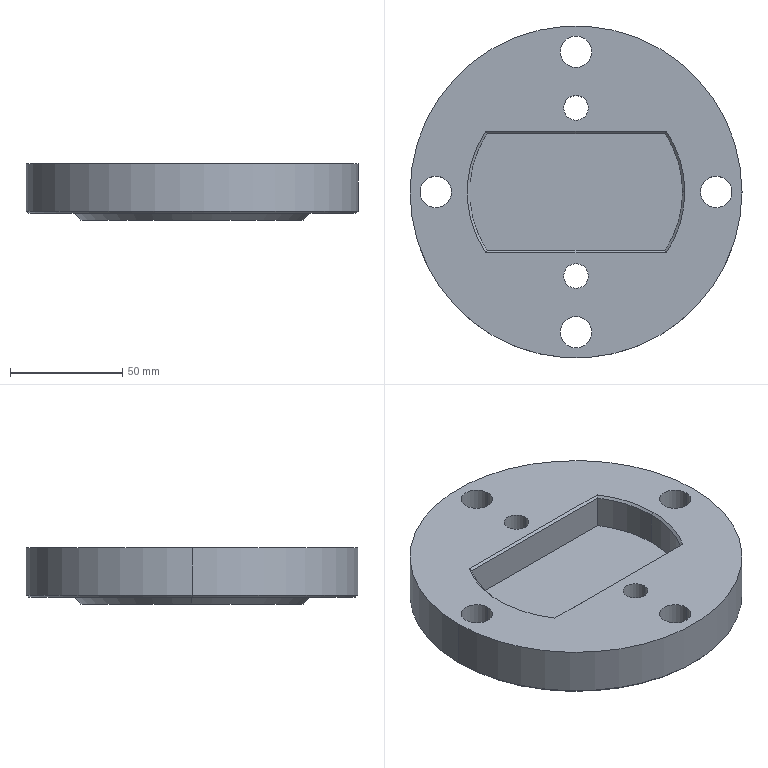Part | SolidWorks | features Chamfer 3, ICE 3, 3DProfileFeature 1, Extrusion 1, HoleWzd 1 | 1 solid | 38 faces | box 148 x 148 x 25 mm | volume 305929 mm3 | cylinder 21 | plane 10 | cone 7 | commonest cylinder face diameters 14 x8 11 x4 18 x4 95 x3 148 x2
STEP:
#1=CARTESIAN_POINT('',(47.5,0.,24.));
#2=VERTEX_POINT('',#1);
#3=CARTESIAN_POINT('',(39.752,26.,24.));
#4=VERTEX_POINT('',#3);
#5=CARTESIAN_POINT('',(0.,0.,24.));
#6=DIRECTION('',(0.,0.,1.));
#7=DIRECTION('',(1.,0.,0.));
#8=AXIS2_PLACEMENT_3D('',#5,#6,#7);
#9=CIRCLE('',#8,47.5);
#10=EDGE_CURVE('',#2,#4,#9,.T.);
#11=ORIENTED_EDGE('',*,*,#10,.F.);
#12=CARTESIAN_POINT('',(48.5,0.,25.));
#13=VERTEX_POINT('',#12);
#14=CARTESIAN_POINT('',(47.5,0.,24.));
#15=DIRECTION('',(0.7071,0.,0.7071));
#16=VECTOR('',#15,1000.);
#17=LINE('',#14,#16);
#18=EDGE_CURVE('',#2,#13,#17,.T.);
#19=ORIENTED_EDGE('',*,*,#18,.T.);
#20=CARTESIAN_POINT('',(40.29,27.,25.));
#21=VERTEX_POINT('',#20);
#22=CARTESIAN_POINT('',(0.,0.,25.));
#23=DIRECTION('',(0.,0.,-1.));
#24=DIRECTION('',(1.,0.,0.));
#25=AXIS2_PLACEMENT_3D('',#22,#23,#24);
#26=CIRCLE('',#25,48.5);
#27=EDGE_CURVE('',#21,#13,#26,.T.);
#28=ORIENTED_EDGE('',*,*,#27,.F.);
#29=CARTESIAN_POINT('',(40.29,27.,25.));
#30=CARTESIAN_POINT('',(40.112,26.666,24.666));
#31=CARTESIAN_POINT('',(39.932,26.333,24.333));
#32=CARTESIAN_POINT('',(39.752,26.,24.));
#33=B_SPLINE_CURVE_WITH_KNOTS('',3,(#29,#30,#31,#32),.UNSPECIFIED.,.F.,.F.,(4,4),(0.,0.001513),.UNSPECIFIED.);
#34=EDGE_CURVE('',#21,#4,#33,.T.);
#35=ORIENTED_EDGE('',*,*,#34,.T.);
#36=EDGE_LOOP('',(#11,#19,#28,#35));
#37=FACE_OUTER_BOUND('',#36,.T.);
#38=CARTESIAN_POINT('',(0.,0.,24.));
#39=DIRECTION('',(0.,0.,1.));
#40=DIRECTION('',(1.,0.,0.));
#41=AXIS2_PLACEMENT_3D('',#38,#39,#40);
#42=CONICAL_SURFACE('',#41,47.5,0.7854);
#43=ADVANCED_FACE('',(#37),#42,.F.);
#44=CARTESIAN_POINT('',(9.,37.5,11.));
#45=VERTEX_POINT('',#44);
#46=CARTESIAN_POINT('',(-9.,37.5,11.));
#47=VERTEX_POINT('',#46);
#48=CARTESIAN_POINT('',(0.,37.5,11.));
#49=DIRECTION('',(0.,0.,-1.));
#50=DIRECTION('',(-1.,0.,0.));
#51=AXIS2_PLACEMENT_3D('',#48,#49,#50);
#52=CIRCLE('',#51,9.);
#53=EDGE_CURVE('',#45,#47,#52,.T.);
#54=ORIENTED_EDGE('',*,*,#53,.F.);
#55=CARTESIAN_POINT('',(9.,37.5,0.));
#56=VERTEX_POINT('',#55);
#57=CARTESIAN_POINT('',(9.,37.5,0.));
#58=DIRECTION('',(0.,0.,-1.));
#59=VECTOR('',#58,1000.);
#60=LINE('',#57,#59);
#61=EDGE_CURVE('',#45,#56,#60,.T.);
#62=ORIENTED_EDGE('',*,*,#61,.T.);
#63=CARTESIAN_POINT('',(-9.,37.5,0.));
#64=VERTEX_POINT('',#63);
#65=CARTESIAN_POINT('',(0.,37.5,0.));
#66=DIRECTION('',(0.,0.,-1.));
#67=DIRECTION('',(-1.,0.,0.));
#68=AXIS2_PLACEMENT_3D('',#65,#66,#67);
#69=CIRCLE('',#68,9.);
#70=EDGE_CURVE('',#56,#64,#69,.T.);
#71=ORIENTED_EDGE('',*,*,#70,.T.);
#72=CARTESIAN_POINT('',(-9.,37.5,0.));
#73=DIRECTION('',(0.,0.,-1.));
#74=VECTOR('',#73,1000.);
#75=LINE('',#72,#74);
#76=EDGE_CURVE('',#47,#64,#75,.T.);
#77=ORIENTED_EDGE('',*,*,#76,.F.);
#78=EDGE_LOOP('',(#54,#62,#71,#77));
#79=FACE_OUTER_BOUND('',#78,.T.);
#80=CARTESIAN_POINT('',(0.,37.5,0.));
#81=DIRECTION('',(0.,0.,-1.));
#82=DIRECTION('',(-1.,0.,0.));
#83=AXIS2_PLACEMENT_3D('',#80,#81,#82);
#84=CYLINDRICAL_SURFACE('',#83,9.);
#85=ADVANCED_FACE('',(#79),#84,.F.);
#86=CARTESIAN_POINT('',(5.5,37.5,25.));
#87=VERTEX_POINT('',#86);
#88=CARTESIAN_POINT('',(-5.5,37.5,25.));
#89=VERTEX_POINT('',#88);
#90=CARTESIAN_POINT('',(0.,37.5,25.));
#91=DIRECTION('',(0.,0.,-1.));
#92=DIRECTION('',(-1.,0.,0.));
#93=AXIS2_PLACEMENT_3D('',#90,#91,#92);
#94=CIRCLE('',#93,5.5);
#95=EDGE_CURVE('',#87,#89,#94,.T.);
#96=ORIENTED_EDGE('',*,*,#95,.F.);
#97=CARTESIAN_POINT('',(5.5,37.5,11.));
#98=VERTEX_POINT('',#97);
#99=CARTESIAN_POINT('',(5.5,37.5,0.));
#100=DIRECTION('',(0.,0.,-1.));
#101=VECTOR('',#100,1000.);
#102=LINE('',#99,#101);
#103=EDGE_CURVE('',#87,#98,#102,.T.);
#104=ORIENTED_EDGE('',*,*,#103,.T.);
#105=CARTESIAN_POINT('',(-5.5,37.5,11.));
#106=VERTEX_POINT('',#105);
#107=CARTESIAN_POINT('',(0.,37.5,11.));
#108=DIRECTION('',(0.,0.,-1.));
#109=DIRECTION('',(-1.,0.,0.));
#110=AXIS2_PLACEMENT_3D('',#107,#108,#109);
#111=CIRCLE('',#110,5.5);
#112=EDGE_CURVE('',#98,#106,#111,.T.);
#113=ORIENTED_EDGE('',*,*,#112,.T.);
#114=CARTESIAN_POINT('',(-5.5,37.5,0.));
#115=DIRECTION('',(0.,0.,-1.));
#116=VECTOR('',#115,1000.);
#117=LINE('',#114,#116);
#118=EDGE_CURVE('',#89,#106,#117,.T.);
#119=ORIENTED_EDGE('',*,*,#118,.F.);
#120=EDGE_LOOP('',(#96,#104,#113,#119));
#121=FACE_OUTER_BOUND('',#120,.T.);
#122=CARTESIAN_POINT('',(0.,37.5,0.));
#123=DIRECTION('',(0.,0.,-1.));
#124=DIRECTION('',(-1.,0.,0.));
#125=AXIS2_PLACEMENT_3D('',#122,#123,#124);
#126=CYLINDRICAL_SURFACE('',#125,5.5);
#127=ADVANCED_FACE('',(#121),#126,.F.);
#128=CARTESIAN_POINT('',(9.,-37.5,11.));
#129=VERTEX_POINT('',#128);
#130=CARTESIAN_POINT('',(-9.,-37.5,11.));
#131=VERTEX_POINT('',#130);
#132=CARTESIAN_POINT('',(0.,-37.5,11.));
#133=DIRECTION('',(0.,0.,-1.));
#134=DIRECTION('',(-1.,0.,0.));
#135=AXIS2_PLACEMENT_3D('',#132,#133,#134);
#136=CIRCLE('',#135,9.);
#137=EDGE_CURVE('',#129,#131,#136,.T.);
#138=ORIENTED_EDGE('',*,*,#137,.F.);
#139=CARTESIAN_POINT('',(9.,-37.5,0.));
#140=VERTEX_POINT('',#139);
#141=CARTESIAN_POINT('',(9.,-37.5,0.));
#142=DIRECTION('',(0.,0.,-1.));
#143=VECTOR('',#142,1000.);
#144=LINE('',#141,#143);
#145=EDGE_CURVE('',#129,#140,#144,.T.);
#146=ORIENTED_EDGE('',*,*,#145,.T.);
#147=CARTESIAN_POINT('',(-9.,-37.5,0.));
#148=VERTEX_POINT('',#147);
#149=CARTESIAN_POINT('',(0.,-37.5,0.));
#150=DIRECTION('',(0.,0.,-1.));
#151=DIRECTION('',(-1.,0.,0.));
#152=AXIS2_PLACEMENT_3D('',#149,#150,#151);
#153=CIRCLE('',#152,9.);
#154=EDGE_CURVE('',#140,#148,#153,.T.);
#155=ORIENTED_EDGE('',*,*,#154,.T.);
#156=CARTESIAN_POINT('',(-9.,-37.5,0.));
#157=DIRECTION('',(0.,0.,-1.));
#158=VECTOR('',#157,1000.);
#159=LINE('',#156,#158);
#160=EDGE_CURVE('',#131,#148,#159,.T.);
#161=ORIENTED_EDGE('',*,*,#160,.F.);
#162=EDGE_LOOP('',(#138,#146,#155,#161));
#163=FACE_OUTER_BOUND('',#162,.T.);
#164=CARTESIAN_POINT('',(0.,-37.5,0.));
#165=DIRECTION('',(0.,0.,-1.));
#166=DIRECTION('',(-1.,0.,0.));
#167=AXIS2_PLACEMENT_3D('',#164,#165,#166);
#168=CYLINDRICAL_SURFACE('',#167,9.);
#169=ADVANCED_FACE('',(#163),#168,.F.);
#170=CARTESIAN_POINT('',(5.5,-37.5,25.));
#171=VERTEX_POINT('',#170);
#172=CARTESIAN_POINT('',(-5.5,-37.5,25.));
#173=VERTEX_POINT('',#172);
#174=CARTESIAN_POINT('',(0.,-37.5,25.));
#175=DIRECTION('',(0.,0.,-1.));
#176=DIRECTION('',(-1.,0.,0.));
#177=AXIS2_PLACEMENT_3D('',#174,#175,#176);
#178=CIRCLE('',#177,5.5);
#179=EDGE_CURVE('',#171,#173,#178,.T.);
#180=ORIENTED_EDGE('',*,*,#179,.F.);
#181=CARTESIAN_POINT('',(5.5,-37.5,11.));
#182=VERTEX_POINT('',#181);
#183=CARTESIAN_POINT('',(5.5,-37.5,0.));
#184=DIRECTION('',(0.,0.,-1.));
#185=VECTOR('',#184,1000.);
#186=LINE('',#183,#185);
#187=EDGE_CURVE('',#171,#182,#186,.T.);
#188=ORIENTED_EDGE('',*,*,#187,.T.);
#189=CARTESIAN_POINT('',(-5.5,-37.5,11.));
#190=VERTEX_POINT('',#189);
#191=CARTESIAN_POINT('',(0.,-37.5,11.));
#192=DIRECTION('',(0.,0.,-1.));
#193=DIRECTION('',(-1.,0.,0.));
#194=AXIS2_PLACEMENT_3D('',#191,#192,#193);
#195=CIRCLE('',#194,5.5);
#196=EDGE_CURVE('',#182,#190,#195,.T.);
#197=ORIENTED_EDGE('',*,*,#196,.T.);
#198=CARTESIAN_POINT('',(-5.5,-37.5,0.));
#199=DIRECTION('',(0.,0.,-1.));
#200=VECTOR('',#199,1000.);
#201=LINE('',#198,#200);
#202=EDGE_CURVE('',#173,#190,#201,.T.);
#203=ORIENTED_EDGE('',*,*,#202,.F.);
#204=EDGE_LOOP('',(#180,#188,#197,#203));
#205=FACE_OUTER_BOUND('',#204,.T.);
#206=CARTESIAN_POINT('',(0.,-37.5,0.));
#207=DIRECTION('',(0.,0.,-1.));
#208=DIRECTION('',(-1.,0.,0.));
#209=AXIS2_PLACEMENT_3D('',#206,#207,#208);
#210=CYLINDRICAL_SURFACE('',#209,5.5);
#211=ADVANCED_FACE('',(#205),#210,.F.);
#212=CARTESIAN_POINT('',(47.5,0.,9.));
#213=VERTEX_POINT('',#212);
#214=CARTESIAN_POINT('',(39.752,26.,9.));
#215=VERTEX_POINT('',#214);
#216=CARTESIAN_POINT('',(0.,0.,9.));
#217=DIRECTION('',(0.,0.,1.));
#218=DIRECTION('',(1.,0.,0.));
#219=AXIS2_PLACEMENT_3D('',#216,#217,#218);
#220=CIRCLE('',#219,47.5);
#221=EDGE_CURVE('',#213,#215,#220,.T.);
#222=ORIENTED_EDGE('',*,*,#221,.F.);
#223=CARTESIAN_POINT('',(47.5,0.,9.));
#224=DIRECTION('',(0.,0.,1.));
#225=VECTOR('',#224,1000.);
#226=LINE('',#223,#225);
#227=EDGE_CURVE('',#213,#2,#226,.T.);
#228=ORIENTED_EDGE('',*,*,#227,.T.);
#229=ORIENTED_EDGE('',*,*,#10,.T.);
#230=CARTESIAN_POINT('',(39.752,26.,9.));
#231=DIRECTION('',(0.,0.,1.));
#232=VECTOR('',#231,1000.);
#233=LINE('',#230,#232);
#234=EDGE_CURVE('',#215,#4,#233,.T.);
#235=ORIENTED_EDGE('',*,*,#234,.F.);
#236=EDGE_LOOP('',(#222,#228,#229,#235));
#237=FACE_OUTER_BOUND('',#236,.T.);
#238=CARTESIAN_POINT('',(0.,0.,9.));
#239=DIRECTION('',(0.,0.,1.));
#240=DIRECTION('',(1.,0.,0.));
#241=AXIS2_PLACEMENT_3D('',#238,#239,#240);
#242=CYLINDRICAL_SURFACE('',#241,47.5);
#243=ADVANCED_FACE('',(#237),#242,.F.);
#244=CARTESIAN_POINT('',(-73.,0.,3.));
#245=VERTEX_POINT('',#244);
#246=CARTESIAN_POINT('',(73.,0.,3.));
#247=VERTEX_POINT('',#246);
#248=CARTESIAN_POINT('',(0.,0.,3.));
#249=DIRECTION('',(0.,0.,-1.));
#250=DIRECTION('',(-1.,0.,0.));
#251=AXIS2_PLACEMENT_3D('',#248,#249,#250);
#252=CIRCLE('',#251,73.);
#253=EDGE_CURVE('',#245,#247,#252,.T.);
#254=ORIENTED_EDGE('',*,*,#253,.F.);
#255=CARTESIAN_POINT('',(-74.,0.,4.));
#256=VERTEX_POINT('',#255);
#257=CARTESIAN_POINT('',(-73.,0.,3.));
#258=DIRECTION('',(-0.7071,0.,0.7071));
#259=VECTOR('',#258,1000.);
#260=LINE('',#257,#259);
#261=EDGE_CURVE('',#245,#256,#260,.T.);
#262=ORIENTED_EDGE('',*,*,#261,.T.);
#263=CARTESIAN_POINT('',(74.,0.,4.));
#264=VERTEX_POINT('',#263);
#265=CARTESIAN_POINT('',(0.,0.,4.));
#266=DIRECTION('',(0.,0.,1.));
#267=DIRECTION('',(-1.,0.,0.));
#268=AXIS2_PLACEMENT_3D('',#265,#266,#267);
#269=CIRCLE('',#268,74.);
#270=EDGE_CURVE('',#264,#256,#269,.T.);
#271=ORIENTED_EDGE('',*,*,#270,.F.);
#272=CARTESIAN_POINT('',(73.,0.,3.));
#273=DIRECTION('',(0.7071,0.,0.7071));
#274=VECTOR('',#273,1000.);
#275=LINE('',#272,#274);
#276=EDGE_CURVE('',#247,#264,#275,.T.);
#277=ORIENTED_EDGE('',*,*,#276,.F.);
#278=EDGE_LOOP('',(#254,#262,#271,#277));
#279=FACE_OUTER_BOUND('',#278,.T.);
#280=CARTESIAN_POINT('',(0.,0.,3.));
#281=DIRECTION('',(0.,0.,1.));
#282=DIRECTION('',(1.,0.,0.));
#283=AXIS2_PLACEMENT_3D('',#280,#281,#282);
#284=CONICAL_SURFACE('',#283,73.,0.7854);
#285=ADVANCED_FACE('',(#279),#284,.T.);
#286=CARTESIAN_POINT('',(-49.5,0.,0.));
#287=VERTEX_POINT('',#286);
#288=CARTESIAN_POINT('',(49.5,0.,0.));
#289=VERTEX_POINT('',#288);
#290=CARTESIAN_POINT('',(0.,0.,0.));
#291=DIRECTION('',(0.,0.,-1.));
#292=DIRECTION('',(1.,0.,0.));
#293=AXIS2_PLACEMENT_3D('',#290,#291,#292);
#294=CIRCLE('',#293,49.5);
#295=EDGE_CURVE('',#287,#289,#294,.T.);
#296=ORIENTED_EDGE('',*,*,#295,.F.);
#297=CARTESIAN_POINT('',(-52.5,0.,3.));
#298=VERTEX_POINT('',#297);
#299=CARTESIAN_POINT('',(-49.5,0.,0.));
#300=DIRECTION('',(-0.7071,0.,0.7071));
#301=VECTOR('',#300,1000.);
#302=LINE('',#299,#301);
#303=EDGE_CURVE('',#287,#298,#302,.T.);
#304=ORIENTED_EDGE('',*,*,#303,.T.);
#305=CARTESIAN_POINT('',(52.5,0.,3.));
#306=VERTEX_POINT('',#305);
#307=CARTESIAN_POINT('',(0.,0.,3.));
#308=DIRECTION('',(0.,0.,-1.));
#309=DIRECTION('',(-1.,0.,0.));
#310=AXIS2_PLACEMENT_3D('',#307,#308,#309);
#311=CIRCLE('',#310,52.5);
#312=EDGE_CURVE('',#298,#306,#311,.T.);
#313=ORIENTED_EDGE('',*,*,#312,.T.);
#314=CARTESIAN_POINT('',(49.5,0.,0.));
#315=DIRECTION('',(0.7071,0.,0.7071));
#316=VECTOR('',#315,1000.);
#317=LINE('',#314,#316);
#318=EDGE_CURVE('',#289,#306,#317,.T.);
#319=ORIENTED_EDGE('',*,*,#318,.F.);
#320=EDGE_LOOP('',(#296,#304,#313,#319));
#321=FACE_OUTER_BOUND('',#320,.T.);
#322=CARTESIAN_POINT('',(0.,0.,0.));
#323=DIRECTION('',(0.,0.,1.));
#324=DIRECTION('',(1.,0.,0.));
#325=AXIS2_PLACEMENT_3D('',#322,#323,#324);
#326=CONICAL_SURFACE('',#325,49.5,0.7854);
#327=ADVANCED_FACE('',(#321),#326,.T.);
#328=CARTESIAN_POINT('',(7.,-62.5,25.));
#329=VERTEX_POINT('',#328);
#330=CARTESIAN_POINT('',(-7.,-62.5,25.));
#331=VERTEX_POINT('',#330);
#332=CARTESIAN_POINT('',(0.,-62.5,25.));
#333=DIRECTION('',(0.,0.,-1.));
#334=DIRECTION('',(-1.,0.,0.));
#335=AXIS2_PLACEMENT_3D('',#332,#333,#334);
#336=CIRCLE('',#335,7.);
#337=EDGE_CURVE('',#329,#331,#336,.T.);
#338=ORIENTED_EDGE('',*,*,#337,.F.);
#339=CARTESIAN_POINT('',(7.,-62.5,3.));
#340=VERTEX_POINT('',#339);
#341=CARTESIAN_POINT('',(7.,-62.5,25.));
#342=DIRECTION('',(0.,0.,-1.));
#343=VECTOR('',#342,1000.);
#344=LINE('',#341,#343);
#345=EDGE_CURVE('',#329,#340,#344,.T.);
#346=ORIENTED_EDGE('',*,*,#345,.T.);
#347=CARTESIAN_POINT('',(-7.,-62.5,3.));
#348=VERTEX_POINT('',#347);
#349=CARTESIAN_POINT('',(0.,-62.5,3.));
#350=DIRECTION('',(0.,0.,-1.));
#351=DIRECTION('',(-1.,0.,0.));
#352=AXIS2_PLACEMENT_3D('',#349,#350,#351);
#353=CIRCLE('',#352,7.);
#354=EDGE_CURVE('',#340,#348,#353,.T.);
#355=ORIENTED_EDGE('',*,*,#354,.T.);
#356=CARTESIAN_POINT('',(-7.,-62.5,25.));
#357=DIRECTION('',(0.,0.,-1.));
#358=VECTOR('',#357,1000.);
#359=LINE('',#356,#358);
#360=EDGE_CURVE('',#331,#348,#359,.T.);
#361=ORIENTED_EDGE('',*,*,#360,.F.);
#362=EDGE_LOOP('',(#338,#346,#355,#361));
#363=FACE_OUTER_BOUND('',#362,.T.);
#364=CARTESIAN_POINT('',(0.,-62.5,25.));
#365=DIRECTION('',(0.,0.,-1.));
#366=DIRECTION('',(-1.,0.,0.));
#367=AXIS2_PLACEMENT_3D('',#364,#365,#366);
#368=CYLINDRICAL_SURFACE('',#367,7.);
#369=ADVANCED_FACE('',(#363),#368,.F.);
#370=CARTESIAN_POINT('',(69.5,0.,25.));
#371=VERTEX_POINT('',#370);
#372=CARTESIAN_POINT('',(55.5,0.,25.));
#373=VERTEX_POINT('',#372);
#374=CARTESIAN_POINT('',(62.5,0.,25.));
#375=DIRECTION('',(0.,0.,-1.));
#376=DIRECTION('',(-1.,0.,0.));
#377=AXIS2_PLACEMENT_3D('',#374,#375,#376);
#378=CIRCLE('',#377,7.);
#379=EDGE_CURVE('',#371,#373,#378,.T.);
#380=ORIENTED_EDGE('',*,*,#379,.F.);
#381=CARTESIAN_POINT('',(69.5,0.,3.));
#382=VERTEX_POINT('',#381);
#383=CARTESIAN_POINT('',(69.5,0.,25.));
#384=DIRECTION('',(0.,0.,-1.));
#385=VECTOR('',#384,1000.);
#386=LINE('',#383,#385);
#387=EDGE_CURVE('',#371,#382,#386,.T.);
#388=ORIENTED_EDGE('',*,*,#387,.T.);
#389=CARTESIAN_POINT('',(55.5,0.,3.));
#390=VERTEX_POINT('',#389);
#391=CARTESIAN_POINT('',(62.5,0.,3.));
#392=DIRECTION('',(0.,0.,-1.));
#393=DIRECTION('',(-1.,0.,0.));
#394=AXIS2_PLACEMENT_3D('',#391,#392,#393);
#395=CIRCLE('',#394,7.);
#396=EDGE_CURVE('',#382,#390,#395,.T.);
#397=ORIENTED_EDGE('',*,*,#396,.T.);
#398=CARTESIAN_POINT('',(55.5,0.,25.));
#399=DIRECTION('',(0.,0.,-1.));
#400=VECTOR('',#399,1000.);
#401=LINE('',#398,#400);
#402=EDGE_CURVE('',#373,#390,#401,.T.);
#403=ORIENTED_EDGE('',*,*,#402,.F.);
#404=EDGE_LOOP('',(#380,#388,#397,#403));
#405=FACE_OUTER_BOUND('',#404,.T.);
#406=CARTESIAN_POINT('',(62.5,0.,25.));
#407=DIRECTION('',(0.,0.,-1.));
#408=DIRECTION('',(-1.,0.,0.));
#409=AXIS2_PLACEMENT_3D('',#406,#407,#408);
#410=CYLINDRICAL_SURFACE('',#409,7.);
#411=ADVANCED_FACE('',(#405),#410,.F.);
#412=CARTESIAN_POINT('',(7.,62.5,25.));
#413=VERTEX_POINT('',#412);
#414=CARTESIAN_POINT('',(-7.,62.5,25.));
#415=VERTEX_POINT('',#414);
#416=CARTESIAN_POINT('',(0.,62.5,25.));
#417=DIRECTION('',(0.,0.,-1.));
#418=DIRECTION('',(-1.,0.,0.));
#419=AXIS2_PLACEMENT_3D('',#416,#417,#418);
#420=CIRCLE('',#419,7.);
#421=EDGE_CURVE('',#413,#415,#420,.T.);
#422=ORIENTED_EDGE('',*,*,#421,.F.);
#423=CARTESIAN_POINT('',(7.,62.5,3.));
#424=VERTEX_POINT('',#423);
#425=CARTESIAN_POINT('',(7.,62.5,25.));
#426=DIRECTION('',(0.,0.,-1.));
#427=VECTOR('',#426,1000.);
#428=LINE('',#425,#427);
#429=EDGE_CURVE('',#413,#424,#428,.T.);
#430=ORIENTED_EDGE('',*,*,#429,.T.);
#431=CARTESIAN_POINT('',(-7.,62.5,3.));
#432=VERTEX_POINT('',#431);
#433=CARTESIAN_POINT('',(0.,62.5,3.));
#434=DIRECTION('',(0.,0.,-1.));
#435=DIRECTION('',(-1.,0.,0.));
#436=AXIS2_PLACEMENT_3D('',#433,#434,#435);
#437=CIRCLE('',#436,7.);
#438=EDGE_CURVE('',#424,#432,#437,.T.);
#439=ORIENTED_EDGE('',*,*,#438,.T.);
#440=CARTESIAN_POINT('',(-7.,62.5,25.));
#441=DIRECTION('',(0.,0.,-1.));
#442=VECTOR('',#441,1000.);
#443=LINE('',#440,#442);
#444=EDGE_CURVE('',#415,#432,#443,.T.);
#445=ORIENTED_EDGE('',*,*,#444,.F.);
#446=EDGE_LOOP('',(#422,#430,#439,#445));
#447=FACE_OUTER_BOUND('',#446,.T.);
#448=CARTESIAN_POINT('',(0.,62.5,25.));
#449=DIRECTION('',(0.,0.,-1.));
#450=DIRECTION('',(-1.,0.,0.));
#451=AXIS2_PLACEMENT_3D('',#448,#449,#450);
#452=CYLINDRICAL_SURFACE('',#451,7.);
#453=ADVANCED_FACE('',(#447),#452,.F.);
#454=CARTESIAN_POINT('',(-55.5,0.,25.));
#455=VERTEX_POINT('',#454);
#456=CARTESIAN_POINT('',(-69.5,0.,25.));
#457=VERTEX_POINT('',#456);
#458=CARTESIAN_POINT('',(-62.5,0.,25.));
#459=DIRECTION('',(0.,0.,-1.));
#460=DIRECTION('',(-1.,0.,0.));
#461=AXIS2_PLACEMENT_3D('',#458,#459,#460);
#462=CIRCLE('',#461,7.);
#463=EDGE_CURVE('',#455,#457,#462,.T.);
#464=ORIENTED_EDGE('',*,*,#463,.F.);
#465=CARTESIAN_POINT('',(-55.5,0.,3.));
#466=VERTEX_POINT('',#465);
#467=CARTESIAN_POINT('',(-55.5,0.,25.));
#468=DIRECTION('',(0.,0.,-1.));
#469=VECTOR('',#468,1000.);
#470=LINE('',#467,#469);
#471=EDGE_CURVE('',#455,#466,#470,.T.);
#472=ORIENTED_EDGE('',*,*,#471,.T.);
#473=CARTESIAN_POINT('',(-69.5,0.,3.));
#474=VERTEX_POINT('',#473);
#475=CARTESIAN_POINT('',(-62.5,0.,3.));
#476=DIRECTION('',(0.,0.,-1.));
#477=DIRECTION('',(-1.,0.,0.));
#478=AXIS2_PLACEMENT_3D('',#475,#476,#477);
#479=CIRCLE('',#478,7.);
#480=EDGE_CURVE('',#466,#474,#479,.T.);
#481=ORIENTED_EDGE('',*,*,#480,.T.);
#482=CARTESIAN_POINT('',(-69.5,0.,25.));
#483=DIRECTION('',(0.,0.,-1.));
#484=VECTOR('',#483,1000.);
#485=LINE('',#482,#484);
#486=EDGE_CURVE('',#457,#474,#485,.T.);
#487=ORIENTED_EDGE('',*,*,#486,.F.);
#488=EDGE_LOOP('',(#464,#472,#481,#487));
#489=FACE_OUTER_BOUND('',#488,.T.);
#490=CARTESIAN_POINT('',(-62.5,0.,25.));
#491=DIRECTION('',(0.,0.,-1.));
#492=DIRECTION('',(-1.,0.,0.));
#493=AXIS2_PLACEMENT_3D('',#490,#491,#492);
#494=CYLINDRICAL_SURFACE('',#493,7.);
#495=ADVANCED_FACE('',(#489),#494,.F.);
#496=CARTESIAN_POINT('',(74.,0.,25.));
#497=VERTEX_POINT('',#496);
#498=CARTESIAN_POINT('',(-74.,0.,25.));
#499=VERTEX_POINT('',#498);
#500=CARTESIAN_POINT('',(0.,0.,25.));
#501=DIRECTION('',(0.,0.,1.));
#502=DIRECTION('',(1.,0.,0.));
#503=AXIS2_PLACEMENT_3D('',#500,#501,#502);
#504=CIRCLE('',#503,74.);
#505=EDGE_CURVE('',#497,#499,#504,.T.);
#506=ORIENTED_EDGE('',*,*,#505,.F.);
#507=CARTESIAN_POINT('',(74.,0.,25.));
#508=DIRECTION('',(0.,0.,-1.));
#509=VECTOR('',#508,1000.);
#510=LINE('',#507,#509);
#511=EDGE_CURVE('',#497,#264,#510,.T.);
#512=ORIENTED_EDGE('',*,*,#511,.T.);
#513=ORIENTED_EDGE('',*,*,#270,.T.);
#514=CARTESIAN_POINT('',(-74.,0.,25.));
#515=DIRECTION('',(0.,0.,-1.));
#516=VECTOR('',#515,1000.);
#517=LINE('',#514,#516);
#518=EDGE_CURVE('',#499,#256,#517,.T.);
#519=ORIENTED_EDGE('',*,*,#518,.F.);
#520=EDGE_LOOP('',(#506,#512,#513,#519));
#521=FACE_OUTER_BOUND('',#520,.T.);
#522=CARTESIAN_POINT('',(0.,0.,25.));
#523=DIRECTION('',(0.,0.,-1.));
#524=DIRECTION('',(-1.,0.,0.));
#525=AXIS2_PLACEMENT_3D('',#522,#523,#524);
#526=CYLINDRICAL_SURFACE('',#525,74.);
#527=ADVANCED_FACE('',(#521),#526,.T.);
#528=ORIENTED_EDGE('',*,*,#511,.F.);
#529=CARTESIAN_POINT('',(0.,0.,25.));
#530=DIRECTION('',(0.,0.,1.));
#531=DIRECTION('',(1.,0.,0.));
#532=AXIS2_PLACEMENT_3D('',#529,#530,#531);
#533=CIRCLE('',#532,74.);
#534=EDGE_CURVE('',#499,#497,#533,.T.);
#535=ORIENTED_EDGE('',*,*,#534,.F.);
#536=ORIENTED_EDGE('',*,*,#518,.T.);
#537=CARTESIAN_POINT('',(0.,0.,4.));
#538=DIRECTION('',(0.,0.,1.));
#539=DIRECTION('',(-1.,0.,0.));
#540=AXIS2_PLACEMENT_3D('',#537,#538,#539);
#541=CIRCLE('',#540,74.);
#542=EDGE_CURVE('',#256,#264,#541,.T.);
#543=ORIENTED_EDGE('',*,*,#542,.T.);
#544=EDGE_LOOP('',(#528,#535,#536,#543));
#545=FACE_OUTER_BOUND('',#544,.T.);
#546=CARTESIAN_POINT('',(0.,0.,25.));
#547=DIRECTION('',(0.,0.,-1.));
#548=DIRECTION('',(-1.,0.,0.));
#549=AXIS2_PLACEMENT_3D('',#546,#547,#548);
#550=CYLINDRICAL_SURFACE('',#549,74.);
#551=ADVANCED_FACE('',(#545),#550,.T.);
#552=CARTESIAN_POINT('',(-40.29,27.,25.));
#553=VERTEX_POINT('',#552);
#554=CARTESIAN_POINT('',(39.752,27.,25.));
#555=DIRECTION('',(1.,0.,0.));
#556=VECTOR('',#555,1000.);
#557=LINE('',#554,#556);
#558=EDGE_CURVE('',#553,#21,#557,.T.);
#559=ORIENTED_EDGE('',*,*,#558,.T.);
#560=ORIENTED_EDGE('',*,*,#27,.T.);
#561=CARTESIAN_POINT('',(40.29,-27.,25.));
#562=VERTEX_POINT('',#561);
#563=CARTESIAN_POINT('',(0.,0.,25.));
#564=DIRECTION('',(0.,0.,-1.));
#565=DIRECTION('',(1.,0.,0.));
#566=AXIS2_PLACEMENT_3D('',#563,#564,#565);
#567=CIRCLE('',#566,48.5);
#568=EDGE_CURVE('',#13,#562,#567,.T.);
#569=ORIENTED_EDGE('',*,*,#568,.T.);
#570=CARTESIAN_POINT('',(-40.29,-27.,25.));
#571=VERTEX_POINT('',#570);
#572=CARTESIAN_POINT('',(-39.752,-27.,25.));
#573=DIRECTION('',(-1.,0.,0.));
#574=VECTOR('',#573,1000.);
#575=LINE('',#572,#574);
#576=EDGE_CURVE('',#562,#571,#575,.T.);
#577=ORIENTED_EDGE('',*,*,#576,.T.);
#578=CARTESIAN_POINT('',(0.,0.,25.));
#579=DIRECTION('',(0.,0.,-1.));
#580=DIRECTION('',(1.,0.,0.));
#581=AXIS2_PLACEMENT_3D('',#578,#579,#580);
#582=CIRCLE('',#581,48.5);
#583=EDGE_CURVE('',#571,#553,#582,.T.);
#584=ORIENTED_EDGE('',*,*,#583,.T.);
#585=EDGE_LOOP('',(#559,#560,#569,#577,#584));
#586=FACE_BOUND('',#585,.T.);
#587=CARTESIAN_POINT('',(0.,37.5,25.));
#588=DIRECTION('',(0.,0.,-1.));
#589=DIRECTION('',(-1.,0.,0.));
#590=AXIS2_PLACEMENT_3D('',#587,#588,#589);
#591=CIRCLE('',#590,5.5);
#592=EDGE_CURVE('',#89,#87,#591,.T.);
#593=ORIENTED_EDGE('',*,*,#592,.T.);
#594=ORIENTED_EDGE('',*,*,#95,.T.);
#595=EDGE_LOOP('',(#593,#594));
#596=FACE_BOUND('',#595,.T.);
#597=CARTESIAN_POINT('',(0.,-37.5,25.));
#598=DIRECTION('',(0.,0.,-1.));
#599=DIRECTION('',(-1.,0.,0.));
#600=AXIS2_PLACEMENT_3D('',#597,#598,#599);
#601=CIRCLE('',#600,5.5);
#602=EDGE_CURVE('',#173,#171,#601,.T.);
#603=ORIENTED_EDGE('',*,*,#602,.T.);
#604=ORIENTED_EDGE('',*,*,#179,.T.);
#605=EDGE_LOOP('',(#603,#604));
#606=FACE_BOUND('',#605,.T.);
#607=CARTESIAN_POINT('',(0.,-62.5,25.));
#608=DIRECTION('',(0.,0.,-1.));
#609=DIRECTION('',(-1.,0.,0.));
#610=AXIS2_PLACEMENT_3D('',#607,#608,#609);
#611=CIRCLE('',#610,7.);
#612=EDGE_CURVE('',#331,#329,#611,.T.);
#613=ORIENTED_EDGE('',*,*,#612,.T.);
#614=ORIENTED_EDGE('',*,*,#337,.T.);
#615=EDGE_LOOP('',(#613,#614));
#616=FACE_BOUND('',#615,.T.);
#617=CARTESIAN_POINT('',(62.5,0.,25.));
#618=DIRECTION('',(0.,0.,-1.));
#619=DIRECTION('',(-1.,0.,0.));
#620=AXIS2_PLACEMENT_3D('',#617,#618,#619);
#621=CIRCLE('',#620,7.);
#622=EDGE_CURVE('',#373,#371,#621,.T.);
#623=ORIENTED_EDGE('',*,*,#622,.T.);
#624=ORIENTED_EDGE('',*,*,#379,.T.);
#625=EDGE_LOOP('',(#623,#624));
#626=FACE_BOUND('',#625,.T.);
#627=CARTESIAN_POINT('',(0.,62.5,25.));
#628=DIRECTION('',(0.,0.,-1.));
#629=DIRECTION('',(-1.,0.,0.));
#630=AXIS2_PLACEMENT_3D('',#627,#628,#629);
#631=CIRCLE('',#630,7.);
#632=EDGE_CURVE('',#415,#413,#631,.T.);
#633=ORIENTED_EDGE('',*,*,#632,.T.);
#634=ORIENTED_EDGE('',*,*,#421,.T.);
#635=EDGE_LOOP('',(#633,#634));
#636=FACE_BOUND('',#635,.T.);
#637=CARTESIAN_POINT('',(-62.5,0.,25.));
#638=DIRECTION('',(0.,0.,-1.));
#639=DIRECTION('',(-1.,0.,0.));
#640=AXIS2_PLACEMENT_3D('',#637,#638,#639);
#641=CIRCLE('',#640,7.);
#642=EDGE_CURVE('',#457,#455,#641,.T.);
#643=ORIENTED_EDGE('',*,*,#642,.T.);
#644=ORIENTED_EDGE('',*,*,#463,.T.);
#645=EDGE_LOOP('',(#643,#644));
#646=FACE_BOUND('',#645,.T.);
#647=ORIENTED_EDGE('',*,*,#534,.T.);
#648=ORIENTED_EDGE('',*,*,#505,.T.);
#649=EDGE_LOOP('',(#647,#648));
#650=FACE_OUTER_BOUND('',#649,.T.);
#651=CARTESIAN_POINT('',(0.,0.,25.));
#652=DIRECTION('',(0.,0.,1.));
#653=DIRECTION('',(1.,0.,0.));
#654=AXIS2_PLACEMENT_3D('',#651,#652,#653);
#655=PLANE('',#654);
#656=ADVANCED_FACE('',(#586,#596,#606,#616,#626,#636,#646,#650),#655,.T.);
#657=CARTESIAN_POINT('',(0.,0.,3.));
#658=DIRECTION('',(0.,0.,-1.));
#659=DIRECTION('',(-1.,0.,0.));
#660=AXIS2_PLACEMENT_3D('',#657,#658,#659);
#661=CIRCLE('',#660,73.);
#662=EDGE_CURVE('',#247,#245,#661,.T.);
#663=ORIENTED_EDGE('',*,*,#662,.T.);
#664=ORIENTED_EDGE('',*,*,#253,.T.);
#665=EDGE_LOOP('',(#663,#664));
#666=FACE_OUTER_BOUND('',#665,.T.);
#667=CARTESIAN_POINT('',(0.,-62.5,3.));
#668=DIRECTION('',(0.,0.,-1.));
#669=DIRECTION('',(-1.,0.,0.));
#670=AXIS2_PLACEMENT_3D('',#667,#668,#669);
#671=CIRCLE('',#670,7.);
#672=EDGE_CURVE('',#348,#340,#671,.T.);
#673=ORIENTED_EDGE('',*,*,#672,.F.);
#674=ORIENTED_EDGE('',*,*,#354,.F.);
#675=EDGE_LOOP('',(#673,#674));
#676=FACE_BOUND('',#675,.T.);
#677=CARTESIAN_POINT('',(62.5,0.,3.));
#678=DIRECTION('',(0.,0.,-1.));
#679=DIRECTION('',(-1.,0.,0.));
#680=AXIS2_PLACEMENT_3D('',#677,#678,#679);
#681=CIRCLE('',#680,7.);
#682=EDGE_CURVE('',#390,#382,#681,.T.);
#683=ORIENTED_EDGE('',*,*,#682,.F.);
#684=ORIENTED_EDGE('',*,*,#396,.F.);
#685=EDGE_LOOP('',(#683,#684));
#686=FACE_BOUND('',#685,.T.);
#687=CARTESIAN_POINT('',(0.,62.5,3.));
#688=DIRECTION('',(0.,0.,-1.));
#689=DIRECTION('',(-1.,0.,0.));
#690=AXIS2_PLACEMENT_3D('',#687,#688,#689);
#691=CIRCLE('',#690,7.);
#692=EDGE_CURVE('',#432,#424,#691,.T.);
#693=ORIENTED_EDGE('',*,*,#692,.F.);
#694=ORIENTED_EDGE('',*,*,#438,.F.);
#695=EDGE_LOOP('',(#693,#694));
#696=FACE_BOUND('',#695,.T.);
#697=CARTESIAN_POINT('',(-62.5,0.,3.));
#698=DIRECTION('',(0.,0.,-1.));
#699=DIRECTION('',(-1.,0.,0.));
#700=AXIS2_PLACEMENT_3D('',#697,#698,#699);
#701=CIRCLE('',#700,7.);
#702=EDGE_CURVE('',#474,#466,#701,.T.);
#703=ORIENTED_EDGE('',*,*,#702,.F.);
#704=ORIENTED_EDGE('',*,*,#480,.F.);
#705=EDGE_LOOP('',(#703,#704));
#706=FACE_BOUND('',#705,.T.);
#707=CARTESIAN_POINT('',(0.,0.,3.));
#708=DIRECTION('',(0.,0.,-1.));
#709=DIRECTION('',(-1.,0.,0.));
#710=AXIS2_PLACEMENT_3D('',#707,#708,#709);
#711=CIRCLE('',#710,52.5);
#712=EDGE_CURVE('',#306,#298,#711,.T.);
#713=ORIENTED_EDGE('',*,*,#712,.F.);
#714=ORIENTED_EDGE('',*,*,#312,.F.);
#715=EDGE_LOOP('',(#713,#714));
#716=FACE_BOUND('',#715,.T.);
#717=CARTESIAN_POINT('',(0.,0.,3.));
#718=DIRECTION('',(0.,0.,-1.));
#719=DIRECTION('',(-1.,0.,0.));
#720=AXIS2_PLACEMENT_3D('',#717,#718,#719);
#721=PLANE('',#720);
#722=ADVANCED_FACE('',(#666,#676,#686,#696,#706,#716),#721,.T.);
#723=CARTESIAN_POINT('',(0.,37.5,0.));
#724=DIRECTION('',(0.,0.,-1.));
#725=DIRECTION('',(-1.,0.,0.));
#726=AXIS2_PLACEMENT_3D('',#723,#724,#725);
#727=CIRCLE('',#726,9.);
#728=EDGE_CURVE('',#64,#56,#727,.T.);
#729=ORIENTED_EDGE('',*,*,#728,.F.);
#730=ORIENTED_EDGE('',*,*,#70,.F.);
#731=EDGE_LOOP('',(#729,#730));
#732=FACE_BOUND('',#731,.T.);
#733=CARTESIAN_POINT('',(0.,-37.5,0.));
#734=DIRECTION('',(0.,0.,-1.));
#735=DIRECTION('',(-1.,0.,0.));
#736=AXIS2_PLACEMENT_3D('',#733,#734,#735);
#737=CIRCLE('',#736,9.);
#738=EDGE_CURVE('',#148,#140,#737,.T.);
#739=ORIENTED_EDGE('',*,*,#738,.F.);
#740=ORIENTED_EDGE('',*,*,#154,.F.);
#741=EDGE_LOOP('',(#739,#740));
#742=FACE_BOUND('',#741,.T.);
#743=CARTESIAN_POINT('',(0.,0.,0.));
#744=DIRECTION('',(0.,0.,-1.));
#745=DIRECTION('',(1.,0.,0.));
#746=AXIS2_PLACEMENT_3D('',#743,#744,#745);
#747=CIRCLE('',#746,49.5);
#748=EDGE_CURVE('',#289,#287,#747,.T.);
#749=ORIENTED_EDGE('',*,*,#748,.T.);
#750=ORIENTED_EDGE('',*,*,#295,.T.);
#751=EDGE_LOOP('',(#749,#750));
#752=FACE_OUTER_BOUND('',#751,.T.);
#753=CARTESIAN_POINT('',(0.,0.,0.));
#754=DIRECTION('',(0.,0.,1.));
#755=DIRECTION('',(1.,0.,0.));
#756=AXIS2_PLACEMENT_3D('',#753,#754,#755);
#757=PLANE('',#756);
#758=ADVANCED_FACE('',(#732,#742,#752),#757,.F.);
#759=ORIENTED_EDGE('',*,*,#471,.F.);
#760=ORIENTED_EDGE('',*,*,#642,.F.);
#761=ORIENTED_EDGE('',*,*,#486,.T.);
#762=ORIENTED_EDGE('',*,*,#702,.T.);
#763=EDGE_LOOP('',(#759,#760,#761,#762));
#764=FACE_OUTER_BOUND('',#763,.T.);
#765=CARTESIAN_POINT('',(-62.5,0.,25.));
#766=DIRECTION('',(0.,0.,-1.));
#767=DIRECTION('',(-1.,0.,0.));
#768=AXIS2_PLACEMENT_3D('',#765,#766,#767);
#769=CYLINDRICAL_SURFACE('',#768,7.);
#770=ADVANCED_FACE('',(#764),#769,.F.);
#771=ORIENTED_EDGE('',*,*,#429,.F.);
#772=ORIENTED_EDGE('',*,*,#632,.F.);
#773=ORIENTED_EDGE('',*,*,#444,.T.);
#774=ORIENTED_EDGE('',*,*,#692,.T.);
#775=EDGE_LOOP('',(#771,#772,#773,#774));
#776=FACE_OUTER_BOUND('',#775,.T.);
#777=CARTESIAN_POINT('',(0.,62.5,25.));
#778=DIRECTION('',(0.,0.,-1.));
#779=DIRECTION('',(-1.,0.,0.));
#780=AXIS2_PLACEMENT_3D('',#777,#778,#779);
#781=CYLINDRICAL_SURFACE('',#780,7.);
#782=ADVANCED_FACE('',(#776),#781,.F.);
#783=ORIENTED_EDGE('',*,*,#387,.F.);
#784=ORIENTED_EDGE('',*,*,#622,.F.);
#785=ORIENTED_EDGE('',*,*,#402,.T.);
#786=ORIENTED_EDGE('',*,*,#682,.T.);
#787=EDGE_LOOP('',(#783,#784,#785,#786));
#788=FACE_OUTER_BOUND('',#787,.T.);
#789=CARTESIAN_POINT('',(62.5,0.,25.));
#790=DIRECTION('',(0.,0.,-1.));
#791=DIRECTION('',(-1.,0.,0.));
#792=AXIS2_PLACEMENT_3D('',#789,#790,#791);
#793=CYLINDRICAL_SURFACE('',#792,7.);
#794=ADVANCED_FACE('',(#788),#793,.F.);
#795=ORIENTED_EDGE('',*,*,#345,.F.);
#796=ORIENTED_EDGE('',*,*,#612,.F.);
#797=ORIENTED_EDGE('',*,*,#360,.T.);
#798=ORIENTED_EDGE('',*,*,#672,.T.);
#799=EDGE_LOOP('',(#795,#796,#797,#798));
#800=FACE_OUTER_BOUND('',#799,.T.);
#801=CARTESIAN_POINT('',(0.,-62.5,25.));
#802=DIRECTION('',(0.,0.,-1.));
#803=DIRECTION('',(-1.,0.,0.));
#804=AXIS2_PLACEMENT_3D('',#801,#802,#803);
#805=CYLINDRICAL_SURFACE('',#804,7.);
#806=ADVANCED_FACE('',(#800),#805,.F.);
#807=ORIENTED_EDGE('',*,*,#303,.F.);
#808=ORIENTED_EDGE('',*,*,#748,.F.);
#809=ORIENTED_EDGE('',*,*,#318,.T.);
#810=ORIENTED_EDGE('',*,*,#712,.T.);
#811=EDGE_LOOP('',(#807,#808,#809,#810));
#812=FACE_OUTER_BOUND('',#811,.T.);
#813=CARTESIAN_POINT('',(0.,0.,0.));
#814=DIRECTION('',(0.,0.,1.));
#815=DIRECTION('',(1.,0.,0.));
#816=AXIS2_PLACEMENT_3D('',#813,#814,#815);
#817=CONICAL_SURFACE('',#816,49.5,0.7854);
#818=ADVANCED_FACE('',(#812),#817,.T.);
#819=ORIENTED_EDGE('',*,*,#261,.F.);
#820=ORIENTED_EDGE('',*,*,#662,.F.);
#821=ORIENTED_EDGE('',*,*,#276,.T.);
#822=ORIENTED_EDGE('',*,*,#542,.F.);
#823=EDGE_LOOP('',(#819,#820,#821,#822));
#824=FACE_OUTER_BOUND('',#823,.T.);
#825=CARTESIAN_POINT('',(0.,0.,3.));
#826=DIRECTION('',(0.,0.,1.));
#827=DIRECTION('',(1.,0.,0.));
#828=AXIS2_PLACEMENT_3D('',#825,#826,#827);
#829=CONICAL_SURFACE('',#828,73.,0.7854);
#830=ADVANCED_FACE('',(#824),#829,.T.);
#831=CARTESIAN_POINT('',(-39.752,26.,9.));
#832=VERTEX_POINT('',#831);
#833=CARTESIAN_POINT('',(-39.752,26.,24.));
#834=VERTEX_POINT('',#833);
#835=CARTESIAN_POINT('',(-39.752,26.,9.));
#836=DIRECTION('',(0.,0.,1.));
#837=VECTOR('',#836,1000.);
#838=LINE('',#835,#837);
#839=EDGE_CURVE('',#832,#834,#838,.T.);
#840=ORIENTED_EDGE('',*,*,#839,.T.);
#841=CARTESIAN_POINT('',(-39.752,-26.,24.));
#842=VERTEX_POINT('',#841);
#843=CARTESIAN_POINT('',(0.,0.,24.));
#844=DIRECTION('',(0.,0.,1.));
#845=DIRECTION('',(1.,0.,0.));
#846=AXIS2_PLACEMENT_3D('',#843,#844,#845);
#847=CIRCLE('',#846,47.5);
#848=EDGE_CURVE('',#834,#842,#847,.T.);
#849=ORIENTED_EDGE('',*,*,#848,.T.);
#850=CARTESIAN_POINT('',(-39.752,-26.,9.));
#851=VERTEX_POINT('',#850);
#852=CARTESIAN_POINT('',(-39.752,-26.,9.));
#853=DIRECTION('',(0.,0.,1.));
#854=VECTOR('',#853,1000.);
#855=LINE('',#852,#854);
#856=EDGE_CURVE('',#851,#842,#855,.T.);
#857=ORIENTED_EDGE('',*,*,#856,.F.);
#858=CARTESIAN_POINT('',(0.,0.,9.));
#859=DIRECTION('',(0.,0.,1.));
#860=DIRECTION('',(1.,0.,0.));
#861=AXIS2_PLACEMENT_3D('',#858,#859,#860);
#862=CIRCLE('',#861,47.5);
#863=EDGE_CURVE('',#832,#851,#862,.T.);
#864=ORIENTED_EDGE('',*,*,#863,.F.);
#865=EDGE_LOOP('',(#840,#849,#857,#864));
#866=FACE_OUTER_BOUND('',#865,.T.);
#867=CARTESIAN_POINT('',(0.,0.,9.));
#868=DIRECTION('',(0.,0.,1.));
#869=DIRECTION('',(1.,0.,0.));
#870=AXIS2_PLACEMENT_3D('',#867,#868,#869);
#871=CYLINDRICAL_SURFACE('',#870,47.5);
#872=ADVANCED_FACE('',(#866),#871,.F.);
#873=ORIENTED_EDGE('',*,*,#234,.T.);
#874=CARTESIAN_POINT('',(-39.752,26.,24.));
#875=DIRECTION('',(-1.,0.,0.));
#876=VECTOR('',#875,1000.);
#877=LINE('',#874,#876);
#878=EDGE_CURVE('',#4,#834,#877,.T.);
#879=ORIENTED_EDGE('',*,*,#878,.T.);
#880=ORIENTED_EDGE('',*,*,#839,.F.);
#881=CARTESIAN_POINT('',(-39.752,26.,9.));
#882=DIRECTION('',(-1.,0.,0.));
#883=VECTOR('',#882,1000.);
#884=LINE('',#881,#883);
#885=EDGE_CURVE('',#215,#832,#884,.T.);
#886=ORIENTED_EDGE('',*,*,#885,.F.);
#887=EDGE_LOOP('',(#873,#879,#880,#886));
#888=FACE_OUTER_BOUND('',#887,.T.);
#889=CARTESIAN_POINT('',(-39.752,26.,9.));
#890=DIRECTION('',(0.,1.,0.));
#891=DIRECTION('',(0.,0.,1.));
#892=AXIS2_PLACEMENT_3D('',#889,#890,#891);
#893=PLANE('',#892);
#894=ADVANCED_FACE('',(#888),#893,.F.);
#895=ORIENTED_EDGE('',*,*,#227,.F.);
#896=CARTESIAN_POINT('',(39.752,-26.,9.));
#897=VERTEX_POINT('',#896);
#898=CARTESIAN_POINT('',(0.,0.,9.));
#899=DIRECTION('',(0.,0.,1.));
#900=DIRECTION('',(1.,0.,0.));
#901=AXIS2_PLACEMENT_3D('',#898,#899,#900);
#902=CIRCLE('',#901,47.5);
#903=EDGE_CURVE('',#897,#213,#902,.T.);
#904=ORIENTED_EDGE('',*,*,#903,.F.);
#905=CARTESIAN_POINT('',(39.752,-26.,24.));
#906=VERTEX_POINT('',#905);
#907=CARTESIAN_POINT('',(39.752,-26.,9.));
#908=DIRECTION('',(0.,0.,1.));
#909=VECTOR('',#908,1000.);
#910=LINE('',#907,#909);
#911=EDGE_CURVE('',#897,#906,#910,.T.);
#912=ORIENTED_EDGE('',*,*,#911,.T.);
#913=CARTESIAN_POINT('',(0.,0.,24.));
#914=DIRECTION('',(0.,0.,1.));
#915=DIRECTION('',(1.,0.,0.));
#916=AXIS2_PLACEMENT_3D('',#913,#914,#915);
#917=CIRCLE('',#916,47.5);
#918=EDGE_CURVE('',#906,#2,#917,.T.);
#919=ORIENTED_EDGE('',*,*,#918,.T.);
#920=EDGE_LOOP('',(#895,#904,#912,#919));
#921=FACE_OUTER_BOUND('',#920,.T.);
#922=CARTESIAN_POINT('',(0.,0.,9.));
#923=DIRECTION('',(0.,0.,1.));
#924=DIRECTION('',(1.,0.,0.));
#925=AXIS2_PLACEMENT_3D('',#922,#923,#924);
#926=CYLINDRICAL_SURFACE('',#925,47.5);
#927=ADVANCED_FACE('',(#921),#926,.F.);
#928=ORIENTED_EDGE('',*,*,#856,.T.);
#929=CARTESIAN_POINT('',(39.752,-26.,24.));
#930=DIRECTION('',(1.,0.,0.));
#931=VECTOR('',#930,1000.);
#932=LINE('',#929,#931);
#933=EDGE_CURVE('',#842,#906,#932,.T.);
#934=ORIENTED_EDGE('',*,*,#933,.T.);
#935=ORIENTED_EDGE('',*,*,#911,.F.);
#936=CARTESIAN_POINT('',(-39.752,-26.,9.));
#937=DIRECTION('',(1.,0.,0.));
#938=VECTOR('',#937,1000.);
#939=LINE('',#936,#938);
#940=EDGE_CURVE('',#851,#897,#939,.T.);
#941=ORIENTED_EDGE('',*,*,#940,.F.);
#942=EDGE_LOOP('',(#928,#934,#935,#941));
#943=FACE_OUTER_BOUND('',#942,.T.);
#944=CARTESIAN_POINT('',(-39.752,-26.,9.));
#945=DIRECTION('',(0.,-1.,0.));
#946=DIRECTION('',(0.,0.,-1.));
#947=AXIS2_PLACEMENT_3D('',#944,#945,#946);
#948=PLANE('',#947);
#949=ADVANCED_FACE('',(#943),#948,.F.);
#950=ORIENTED_EDGE('',*,*,#863,.T.);
#951=ORIENTED_EDGE('',*,*,#940,.T.);
#952=ORIENTED_EDGE('',*,*,#903,.T.);
#953=ORIENTED_EDGE('',*,*,#221,.T.);
#954=ORIENTED_EDGE('',*,*,#885,.T.);
#955=EDGE_LOOP('',(#950,#951,#952,#953,#954));
#956=FACE_OUTER_BOUND('',#955,.T.);
#957=CARTESIAN_POINT('',(0.,0.,9.));
#958=DIRECTION('',(0.,0.,1.));
#959=DIRECTION('',(1.,0.,0.));
#960=AXIS2_PLACEMENT_3D('',#957,#958,#959);
#961=PLANE('',#960);
#962=ADVANCED_FACE('',(#956),#961,.T.);
#963=ORIENTED_EDGE('',*,*,#187,.F.);
#964=ORIENTED_EDGE('',*,*,#602,.F.);
#965=ORIENTED_EDGE('',*,*,#202,.T.);
#966=CARTESIAN_POINT('',(0.,-37.5,11.));
#967=DIRECTION('',(0.,0.,-1.));
#968=DIRECTION('',(-1.,0.,0.));
#969=AXIS2_PLACEMENT_3D('',#966,#967,#968);
#970=CIRCLE('',#969,5.5);
#971=EDGE_CURVE('',#190,#182,#970,.T.);
#972=ORIENTED_EDGE('',*,*,#971,.T.);
#973=EDGE_LOOP('',(#963,#964,#965,#972));
#974=FACE_OUTER_BOUND('',#973,.T.);
#975=CARTESIAN_POINT('',(0.,-37.5,0.));
#976=DIRECTION('',(0.,0.,-1.));
#977=DIRECTION('',(-1.,0.,0.));
#978=AXIS2_PLACEMENT_3D('',#975,#976,#977);
#979=CYLINDRICAL_SURFACE('',#978,5.5);
#980=ADVANCED_FACE('',(#974),#979,.F.);
#981=ORIENTED_EDGE('',*,*,#971,.F.);
#982=ORIENTED_EDGE('',*,*,#196,.F.);
#983=EDGE_LOOP('',(#981,#982));
#984=FACE_BOUND('',#983,.T.);
#985=CARTESIAN_POINT('',(0.,-37.5,11.));
#986=DIRECTION('',(0.,0.,-1.));
#987=DIRECTION('',(-1.,0.,0.));
#988=AXIS2_PLACEMENT_3D('',#985,#986,#987);
#989=CIRCLE('',#988,9.);
#990=EDGE_CURVE('',#131,#129,#989,.T.);
#991=ORIENTED_EDGE('',*,*,#990,.T.);
#992=ORIENTED_EDGE('',*,*,#137,.T.);
#993=EDGE_LOOP('',(#991,#992));
#994=FACE_OUTER_BOUND('',#993,.T.);
#995=CARTESIAN_POINT('',(5.5,-37.5,11.));
#996=DIRECTION('',(0.,0.,1.));
#997=DIRECTION('',(1.,0.,0.));
#998=AXIS2_PLACEMENT_3D('',#995,#996,#997);
#999=PLANE('',#998);
#1000=ADVANCED_FACE('',(#984,#994),#999,.F.);
#1001=ORIENTED_EDGE('',*,*,#145,.F.);
#1002=ORIENTED_EDGE('',*,*,#990,.F.);
#1003=ORIENTED_EDGE('',*,*,#160,.T.);
#1004=ORIENTED_EDGE('',*,*,#738,.T.);
#1005=EDGE_LOOP('',(#1001,#1002,#1003,#1004));
#1006=FACE_OUTER_BOUND('',#1005,.T.);
#1007=CARTESIAN_POINT('',(0.,-37.5,0.));
#1008=DIRECTION('',(0.,0.,-1.));
#1009=DIRECTION('',(-1.,0.,0.));
#1010=AXIS2_PLACEMENT_3D('',#1007,#1008,#1009);
#1011=CYLINDRICAL_SURFACE('',#1010,9.);
#1012=ADVANCED_FACE('',(#1006),#1011,.F.);
#1013=ORIENTED_EDGE('',*,*,#103,.F.);
#1014=ORIENTED_EDGE('',*,*,#592,.F.);
#1015=ORIENTED_EDGE('',*,*,#118,.T.);
#1016=CARTESIAN_POINT('',(0.,37.5,11.));
#1017=DIRECTION('',(0.,0.,-1.));
#1018=DIRECTION('',(-1.,0.,0.));
#1019=AXIS2_PLACEMENT_3D('',#1016,#1017,#1018);
#1020=CIRCLE('',#1019,5.5);
#1021=EDGE_CURVE('',#106,#98,#1020,.T.);
#1022=ORIENTED_EDGE('',*,*,#1021,.T.);
#1023=EDGE_LOOP('',(#1013,#1014,#1015,#1022));
#1024=FACE_OUTER_BOUND('',#1023,.T.);
#1025=CARTESIAN_POINT('',(0.,37.5,0.));
#1026=DIRECTION('',(0.,0.,-1.));
#1027=DIRECTION('',(-1.,0.,0.));
#1028=AXIS2_PLACEMENT_3D('',#1025,#1026,#1027);
#1029=CYLINDRICAL_SURFACE('',#1028,5.5);
#1030=ADVANCED_FACE('',(#1024),#1029,.F.);
#1031=ORIENTED_EDGE('',*,*,#1021,.F.);
#1032=ORIENTED_EDGE('',*,*,#112,.F.);
#1033=EDGE_LOOP('',(#1031,#1032));
#1034=FACE_BOUND('',#1033,.T.);
#1035=CARTESIAN_POINT('',(0.,37.5,11.));
#1036=DIRECTION('',(0.,0.,-1.));
#1037=DIRECTION('',(-1.,0.,0.));
#1038=AXIS2_PLACEMENT_3D('',#1035,#1036,#1037);
#1039=CIRCLE('',#1038,9.);
#1040=EDGE_CURVE('',#47,#45,#1039,.T.);
#1041=ORIENTED_EDGE('',*,*,#1040,.T.);
#1042=ORIENTED_EDGE('',*,*,#53,.T.);
#1043=EDGE_LOOP('',(#1041,#1042));
#1044=FACE_OUTER_BOUND('',#1043,.T.);
#1045=CARTESIAN_POINT('',(5.5,37.5,11.));
#1046=DIRECTION('',(0.,0.,1.));
#1047=DIRECTION('',(1.,0.,0.));
#1048=AXIS2_PLACEMENT_3D('',#1045,#1046,#1047);
#1049=PLANE('',#1048);
#1050=ADVANCED_FACE('',(#1034,#1044),#1049,.F.);
#1051=ORIENTED_EDGE('',*,*,#61,.F.);
#1052=ORIENTED_EDGE('',*,*,#1040,.F.);
#1053=ORIENTED_EDGE('',*,*,#76,.T.);
#1054=ORIENTED_EDGE('',*,*,#728,.T.);
#1055=EDGE_LOOP('',(#1051,#1052,#1053,#1054));
#1056=FACE_OUTER_BOUND('',#1055,.T.);
#1057=CARTESIAN_POINT('',(0.,37.5,0.));
#1058=DIRECTION('',(0.,0.,-1.));
#1059=DIRECTION('',(-1.,0.,0.));
#1060=AXIS2_PLACEMENT_3D('',#1057,#1058,#1059);
#1061=CYLINDRICAL_SURFACE('',#1060,9.);
#1062=ADVANCED_FACE('',(#1056),#1061,.F.);
#1063=CARTESIAN_POINT('',(-40.29,27.,25.));
#1064=CARTESIAN_POINT('',(-40.112,26.666,24.666));
#1065=CARTESIAN_POINT('',(-39.932,26.333,24.333));
#1066=CARTESIAN_POINT('',(-39.752,26.,24.));
#1067=B_SPLINE_CURVE_WITH_KNOTS('',3,(#1063,#1064,#1065,#1066),.UNSPECIFIED.,.F.,.F.,(4,4),(0.,0.001513),.UNSPECIFIED.);
#1068=EDGE_CURVE('',#553,#834,#1067,.T.);
#1069=ORIENTED_EDGE('',*,*,#1068,.F.);
#1070=ORIENTED_EDGE('',*,*,#583,.F.);
#1071=CARTESIAN_POINT('',(-39.752,-26.,24.));
#1072=CARTESIAN_POINT('',(-39.932,-26.333,24.333));
#1073=CARTESIAN_POINT('',(-40.112,-26.666,24.666));
#1074=CARTESIAN_POINT('',(-40.29,-27.,25.));
#1075=B_SPLINE_CURVE_WITH_KNOTS('',3,(#1071,#1072,#1073,#1074),.UNSPECIFIED.,.F.,.F.,(4,4),(0.,0.001513),.UNSPECIFIED.);
#1076=EDGE_CURVE('',#842,#571,#1075,.T.);
#1077=ORIENTED_EDGE('',*,*,#1076,.F.);
#1078=ORIENTED_EDGE('',*,*,#848,.F.);
#1079=EDGE_LOOP('',(#1069,#1070,#1077,#1078));
#1080=FACE_OUTER_BOUND('',#1079,.T.);
#1081=CARTESIAN_POINT('',(0.,0.,24.));
#1082=DIRECTION('',(0.,0.,1.));
#1083=DIRECTION('',(1.,0.,0.));
#1084=AXIS2_PLACEMENT_3D('',#1081,#1082,#1083);
#1085=CONICAL_SURFACE('',#1084,47.5,0.7854);
#1086=ADVANCED_FACE('',(#1080),#1085,.F.);
#1087=ORIENTED_EDGE('',*,*,#1076,.T.);
#1088=ORIENTED_EDGE('',*,*,#576,.F.);
#1089=CARTESIAN_POINT('',(39.752,-26.,24.));
#1090=CARTESIAN_POINT('',(39.932,-26.333,24.333));
#1091=CARTESIAN_POINT('',(40.112,-26.666,24.666));
#1092=CARTESIAN_POINT('',(40.29,-27.,25.));
#1093=B_SPLINE_CURVE_WITH_KNOTS('',3,(#1089,#1090,#1091,#1092),.UNSPECIFIED.,.F.,.F.,(4,4),(0.,0.001513),.UNSPECIFIED.);
#1094=EDGE_CURVE('',#906,#562,#1093,.T.);
#1095=ORIENTED_EDGE('',*,*,#1094,.F.);
#1096=ORIENTED_EDGE('',*,*,#933,.F.);
#1097=EDGE_LOOP('',(#1087,#1088,#1095,#1096));
#1098=FACE_OUTER_BOUND('',#1097,.T.);
#1099=CARTESIAN_POINT('',(-39.752,-26.,24.));
#1100=DIRECTION('',(0.,0.7071,0.7071));
#1101=DIRECTION('',(-1.,0.,0.));
#1102=AXIS2_PLACEMENT_3D('',#1099,#1100,#1101);
#1103=PLANE('',#1102);
#1104=ADVANCED_FACE('',(#1098),#1103,.T.);
#1105=ORIENTED_EDGE('',*,*,#1068,.T.);
#1106=ORIENTED_EDGE('',*,*,#878,.F.);
#1107=ORIENTED_EDGE('',*,*,#34,.F.);
#1108=ORIENTED_EDGE('',*,*,#558,.F.);
#1109=EDGE_LOOP('',(#1105,#1106,#1107,#1108));
#1110=FACE_OUTER_BOUND('',#1109,.T.);
#1111=CARTESIAN_POINT('',(-39.752,26.,24.));
#1112=DIRECTION('',(0.,-0.7071,0.7071));
#1113=DIRECTION('',(1.,0.,0.));
#1114=AXIS2_PLACEMENT_3D('',#1111,#1112,#1113);
#1115=PLANE('',#1114);
#1116=ADVANCED_FACE('',(#1110),#1115,.T.);
#1117=ORIENTED_EDGE('',*,*,#18,.F.);
#1118=ORIENTED_EDGE('',*,*,#918,.F.);
#1119=ORIENTED_EDGE('',*,*,#1094,.T.);
#1120=ORIENTED_EDGE('',*,*,#568,.F.);
#1121=EDGE_LOOP('',(#1117,#1118,#1119,#1120));
#1122=FACE_OUTER_BOUND('',#1121,.T.);
#1123=CARTESIAN_POINT('',(0.,0.,24.));
#1124=DIRECTION('',(0.,0.,1.));
#1125=DIRECTION('',(1.,0.,0.));
#1126=AXIS2_PLACEMENT_3D('',#1123,#1124,#1125);
#1127=CONICAL_SURFACE('',#1126,47.5,0.7854);
#1128=ADVANCED_FACE('',(#1122),#1127,.F.);
#1129=CLOSED_SHELL('',(#43,#85,#127,#169,#211,#243,#285,#327,#369,#411,#453,#495,#527,#551,#656,#722,#758,#770,#782,#794,#806,#818,#830,#872,#894,#927,#949,#962,#980,#1000,#1012,#1030,#1050,#1062,#1086,#1104,#1116,#1128));
#1130=MANIFOLD_SOLID_BREP('',#1129);
#1131=CARTESIAN_POINT('',(0.,0.,0.));
#1132=DIRECTION('',(0.,0.,1.));
#1133=DIRECTION('',(1.,0.,0.));
#1134=AXIS2_PLACEMENT_3D('',#1131,#1132,#1133);
#1135=(LENGTH_UNIT()NAMED_UNIT(*)SI_UNIT(.MILLI.,.METRE.));
#1136=UNCERTAINTY_MEASURE_WITH_UNIT(LENGTH_MEASURE(0.00001),#1135,'','');
#1137=(NAMED_UNIT(*)PLANE_ANGLE_UNIT()SI_UNIT($,.RADIAN.));
#1138=(NAMED_UNIT(*)SI_UNIT($,.STERADIAN.)SOLID_ANGLE_UNIT());
#1139=(GEOMETRIC_REPRESENTATION_CONTEXT(3)GLOBAL_UNCERTAINTY_ASSIGNED_CONTEXT((#1136))GLOBAL_UNIT_ASSIGNED_CONTEXT((#1135,#1137,#1138))REPRESENTATION_CONTEXT('',''));
#1140=ADVANCED_BREP_SHAPE_REPRESENTATION('',(#1130,#1134),#1139);